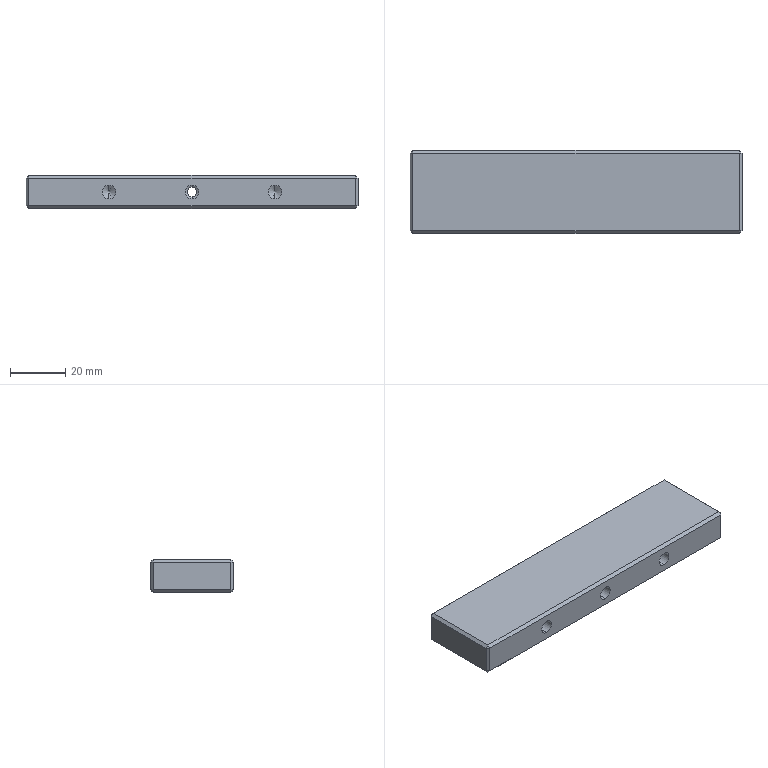Part | STEP file | 03-17 trimming upper support bracket | 1 solid | 50 faces | box 120 x 30 x 12 mm | volume 41120 mm3 | plane 26 | cylinder 12 | cone 12 | commonest cylinder face diameters 5 x12
STEP:
#1=CARTESIAN_POINT('',(35.,1.,3.5));
#2=VERTEX_POINT('',#1);
#3=CARTESIAN_POINT('',(35.,1.,8.5));
#4=VERTEX_POINT('',#3);
#5=CARTESIAN_POINT('',(35.,1.,6.));
#6=DIRECTION('',(0.,1.,0.));
#7=DIRECTION('',(0.,0.,1.));
#8=AXIS2_PLACEMENT_3D('',#5,#6,#7);
#9=CIRCLE('',#8,2.5);
#10=EDGE_CURVE('',#2,#4,#9,.T.);
#11=ORIENTED_EDGE('',*,*,#10,.F.);
#12=CARTESIAN_POINT('',(35.,15.,3.5));
#13=VERTEX_POINT('',#12);
#14=CARTESIAN_POINT('',(35.,15.,3.5));
#15=DIRECTION('',(0.,1.,0.));
#16=VECTOR('',#15,1000.);
#17=LINE('',#14,#16);
#18=EDGE_CURVE('',#2,#13,#17,.T.);
#19=ORIENTED_EDGE('',*,*,#18,.T.);
#20=CARTESIAN_POINT('',(35.,15.,8.5));
#21=VERTEX_POINT('',#20);
#22=CARTESIAN_POINT('',(35.,15.,6.));
#23=DIRECTION('',(0.,1.,0.));
#24=DIRECTION('',(0.,0.,1.));
#25=AXIS2_PLACEMENT_3D('',#22,#23,#24);
#26=CIRCLE('',#25,2.5);
#27=EDGE_CURVE('',#13,#21,#26,.T.);
#28=ORIENTED_EDGE('',*,*,#27,.T.);
#29=CARTESIAN_POINT('',(35.,15.,8.5));
#30=DIRECTION('',(0.,1.,0.));
#31=VECTOR('',#30,1000.);
#32=LINE('',#29,#31);
#33=EDGE_CURVE('',#4,#21,#32,.T.);
#34=ORIENTED_EDGE('',*,*,#33,.F.);
#35=EDGE_LOOP('',(#11,#19,#28,#34));
#36=FACE_OUTER_BOUND('',#35,.T.);
#37=CARTESIAN_POINT('',(35.,15.,6.));
#38=DIRECTION('',(0.,1.,0.));
#39=DIRECTION('',(0.,0.,1.));
#40=AXIS2_PLACEMENT_3D('',#37,#38,#39);
#41=CYLINDRICAL_SURFACE('',#40,2.5);
#42=ADVANCED_FACE('',(#36),#41,.F.);
#43=CARTESIAN_POINT('',(35.,-0.5022,6.));
#44=VERTEX_POINT('',#43);
#45=CARTESIAN_POINT('',(35.,1.,8.5));
#46=DIRECTION('',(0.,0.515,0.8572));
#47=VECTOR('',#46,1000.);
#48=LINE('',#45,#47);
#49=EDGE_CURVE('',#44,#4,#48,.T.);
#50=ORIENTED_EDGE('',*,*,#49,.F.);
#51=CARTESIAN_POINT('',(35.,1.,3.5));
#52=DIRECTION('',(0.,0.515,-0.8572));
#53=VECTOR('',#52,1000.);
#54=LINE('',#51,#53);
#55=EDGE_CURVE('',#44,#2,#54,.T.);
#56=ORIENTED_EDGE('',*,*,#55,.T.);
#57=ORIENTED_EDGE('',*,*,#10,.T.);
#58=EDGE_LOOP('',(#50,#56,#57));
#59=FACE_OUTER_BOUND('',#58,.T.);
#60=CARTESIAN_POINT('',(35.,1.,6.));
#61=DIRECTION('',(0.,1.,0.));
#62=DIRECTION('',(0.,0.,1.));
#63=AXIS2_PLACEMENT_3D('',#60,#61,#62);
#64=CONICAL_SURFACE('',#63,2.5,1.03);
#65=ADVANCED_FACE('',(#59),#64,.F.);
#66=CARTESIAN_POINT('',(0.,1.,3.5));
#67=VERTEX_POINT('',#66);
#68=CARTESIAN_POINT('',(0.,1.,8.5));
#69=VERTEX_POINT('',#68);
#70=CARTESIAN_POINT('',(0.,1.,6.));
#71=DIRECTION('',(0.,1.,0.));
#72=DIRECTION('',(0.,0.,1.));
#73=AXIS2_PLACEMENT_3D('',#70,#71,#72);
#74=CIRCLE('',#73,2.5);
#75=EDGE_CURVE('',#67,#69,#74,.T.);
#76=ORIENTED_EDGE('',*,*,#75,.F.);
#77=CARTESIAN_POINT('',(0.,15.,3.5));
#78=VERTEX_POINT('',#77);
#79=CARTESIAN_POINT('',(0.,15.,3.5));
#80=DIRECTION('',(0.,1.,0.));
#81=VECTOR('',#80,1000.);
#82=LINE('',#79,#81);
#83=EDGE_CURVE('',#67,#78,#82,.T.);
#84=ORIENTED_EDGE('',*,*,#83,.T.);
#85=CARTESIAN_POINT('',(0.,15.,8.5));
#86=VERTEX_POINT('',#85);
#87=CARTESIAN_POINT('',(0.,15.,6.));
#88=DIRECTION('',(0.,1.,0.));
#89=DIRECTION('',(0.,0.,1.));
#90=AXIS2_PLACEMENT_3D('',#87,#88,#89);
#91=CIRCLE('',#90,2.5);
#92=EDGE_CURVE('',#78,#86,#91,.T.);
#93=ORIENTED_EDGE('',*,*,#92,.T.);
#94=CARTESIAN_POINT('',(0.,15.,8.5));
#95=DIRECTION('',(0.,1.,0.));
#96=VECTOR('',#95,1000.);
#97=LINE('',#94,#96);
#98=EDGE_CURVE('',#69,#86,#97,.T.);
#99=ORIENTED_EDGE('',*,*,#98,.F.);
#100=EDGE_LOOP('',(#76,#84,#93,#99));
#101=FACE_OUTER_BOUND('',#100,.T.);
#102=CARTESIAN_POINT('',(0.,15.,6.));
#103=DIRECTION('',(0.,1.,0.));
#104=DIRECTION('',(0.,0.,1.));
#105=AXIS2_PLACEMENT_3D('',#102,#103,#104);
#106=CYLINDRICAL_SURFACE('',#105,2.5);
#107=ADVANCED_FACE('',(#101),#106,.F.);
#108=CARTESIAN_POINT('',(0.,0.5,4.332));
#109=VERTEX_POINT('',#108);
#110=CARTESIAN_POINT('',(0.,0.5,7.668));
#111=VERTEX_POINT('',#110);
#112=CARTESIAN_POINT('',(0.,0.5,6.));
#113=DIRECTION('',(0.,1.,0.));
#114=DIRECTION('',(0.,0.,1.));
#115=AXIS2_PLACEMENT_3D('',#112,#113,#114);
#116=CIRCLE('',#115,1.668);
#117=EDGE_CURVE('',#109,#111,#116,.T.);
#118=ORIENTED_EDGE('',*,*,#117,.F.);
#119=CARTESIAN_POINT('',(0.,1.,3.5));
#120=DIRECTION('',(0.,0.515,-0.8572));
#121=VECTOR('',#120,1000.);
#122=LINE('',#119,#121);
#123=EDGE_CURVE('',#109,#67,#122,.T.);
#124=ORIENTED_EDGE('',*,*,#123,.T.);
#125=ORIENTED_EDGE('',*,*,#75,.T.);
#126=CARTESIAN_POINT('',(0.,1.,8.5));
#127=DIRECTION('',(0.,0.515,0.8572));
#128=VECTOR('',#127,1000.);
#129=LINE('',#126,#128);
#130=EDGE_CURVE('',#111,#69,#129,.T.);
#131=ORIENTED_EDGE('',*,*,#130,.F.);
#132=EDGE_LOOP('',(#118,#124,#125,#131));
#133=FACE_OUTER_BOUND('',#132,.T.);
#134=CARTESIAN_POINT('',(0.,1.,6.));
#135=DIRECTION('',(0.,1.,0.));
#136=DIRECTION('',(0.,0.,1.));
#137=AXIS2_PLACEMENT_3D('',#134,#135,#136);
#138=CONICAL_SURFACE('',#137,2.5,1.03);
#139=ADVANCED_FACE('',(#133),#138,.F.);
#140=CARTESIAN_POINT('',(-35.,1.,3.5));
#141=VERTEX_POINT('',#140);
#142=CARTESIAN_POINT('',(-35.,1.,8.5));
#143=VERTEX_POINT('',#142);
#144=CARTESIAN_POINT('',(-35.,1.,6.));
#145=DIRECTION('',(0.,1.,0.));
#146=DIRECTION('',(0.,0.,1.));
#147=AXIS2_PLACEMENT_3D('',#144,#145,#146);
#148=CIRCLE('',#147,2.5);
#149=EDGE_CURVE('',#141,#143,#148,.T.);
#150=ORIENTED_EDGE('',*,*,#149,.F.);
#151=CARTESIAN_POINT('',(-35.,15.,3.5));
#152=VERTEX_POINT('',#151);
#153=CARTESIAN_POINT('',(-35.,15.,3.5));
#154=DIRECTION('',(0.,1.,0.));
#155=VECTOR('',#154,1000.);
#156=LINE('',#153,#155);
#157=EDGE_CURVE('',#141,#152,#156,.T.);
#158=ORIENTED_EDGE('',*,*,#157,.T.);
#159=CARTESIAN_POINT('',(-35.,15.,8.5));
#160=VERTEX_POINT('',#159);
#161=CARTESIAN_POINT('',(-35.,15.,6.));
#162=DIRECTION('',(0.,1.,0.));
#163=DIRECTION('',(0.,0.,1.));
#164=AXIS2_PLACEMENT_3D('',#161,#162,#163);
#165=CIRCLE('',#164,2.5);
#166=EDGE_CURVE('',#152,#160,#165,.T.);
#167=ORIENTED_EDGE('',*,*,#166,.T.);
#168=CARTESIAN_POINT('',(-35.,15.,8.5));
#169=DIRECTION('',(0.,1.,0.));
#170=VECTOR('',#169,1000.);
#171=LINE('',#168,#170);
#172=EDGE_CURVE('',#143,#160,#171,.T.);
#173=ORIENTED_EDGE('',*,*,#172,.F.);
#174=EDGE_LOOP('',(#150,#158,#167,#173));
#175=FACE_OUTER_BOUND('',#174,.T.);
#176=CARTESIAN_POINT('',(-35.,15.,6.));
#177=DIRECTION('',(0.,1.,0.));
#178=DIRECTION('',(0.,0.,1.));
#179=AXIS2_PLACEMENT_3D('',#176,#177,#178);
#180=CYLINDRICAL_SURFACE('',#179,2.5);
#181=ADVANCED_FACE('',(#175),#180,.F.);
#182=CARTESIAN_POINT('',(-35.,-0.5022,6.));
#183=VERTEX_POINT('',#182);
#184=CARTESIAN_POINT('',(-35.,1.,8.5));
#185=DIRECTION('',(0.,0.515,0.8572));
#186=VECTOR('',#185,1000.);
#187=LINE('',#184,#186);
#188=EDGE_CURVE('',#183,#143,#187,.T.);
#189=ORIENTED_EDGE('',*,*,#188,.F.);
#190=CARTESIAN_POINT('',(-35.,1.,3.5));
#191=DIRECTION('',(0.,0.515,-0.8572));
#192=VECTOR('',#191,1000.);
#193=LINE('',#190,#192);
#194=EDGE_CURVE('',#183,#141,#193,.T.);
#195=ORIENTED_EDGE('',*,*,#194,.T.);
#196=ORIENTED_EDGE('',*,*,#149,.T.);
#197=EDGE_LOOP('',(#189,#195,#196));
#198=FACE_OUTER_BOUND('',#197,.T.);
#199=CARTESIAN_POINT('',(-35.,1.,6.));
#200=DIRECTION('',(0.,1.,0.));
#201=DIRECTION('',(0.,0.,1.));
#202=AXIS2_PLACEMENT_3D('',#199,#200,#201);
#203=CONICAL_SURFACE('',#202,2.5,1.03);
#204=ADVANCED_FACE('',(#198),#203,.F.);
#205=CARTESIAN_POINT('',(30.,0.,8.5));
#206=VERTEX_POINT('',#205);
#207=CARTESIAN_POINT('',(30.,0.,3.5));
#208=VERTEX_POINT('',#207);
#209=CARTESIAN_POINT('',(30.,0.,6.));
#210=DIRECTION('',(0.,-1.,0.));
#211=DIRECTION('',(0.,0.,-1.));
#212=AXIS2_PLACEMENT_3D('',#209,#210,#211);
#213=CIRCLE('',#212,2.5);
#214=EDGE_CURVE('',#206,#208,#213,.T.);
#215=ORIENTED_EDGE('',*,*,#214,.F.);
#216=CARTESIAN_POINT('',(30.,-15.,8.5));
#217=VERTEX_POINT('',#216);
#218=CARTESIAN_POINT('',(30.,-15.,8.5));
#219=DIRECTION('',(0.,-1.,0.));
#220=VECTOR('',#219,1000.);
#221=LINE('',#218,#220);
#222=EDGE_CURVE('',#206,#217,#221,.T.);
#223=ORIENTED_EDGE('',*,*,#222,.T.);
#224=CARTESIAN_POINT('',(30.,-15.,3.5));
#225=VERTEX_POINT('',#224);
#226=CARTESIAN_POINT('',(30.,-15.,6.));
#227=DIRECTION('',(0.,-1.,0.));
#228=DIRECTION('',(0.,0.,-1.));
#229=AXIS2_PLACEMENT_3D('',#226,#227,#228);
#230=CIRCLE('',#229,2.5);
#231=EDGE_CURVE('',#217,#225,#230,.T.);
#232=ORIENTED_EDGE('',*,*,#231,.T.);
#233=CARTESIAN_POINT('',(30.,-15.,3.5));
#234=DIRECTION('',(0.,-1.,0.));
#235=VECTOR('',#234,1000.);
#236=LINE('',#233,#235);
#237=EDGE_CURVE('',#208,#225,#236,.T.);
#238=ORIENTED_EDGE('',*,*,#237,.F.);
#239=EDGE_LOOP('',(#215,#223,#232,#238));
#240=FACE_OUTER_BOUND('',#239,.T.);
#241=CARTESIAN_POINT('',(30.,-15.,6.));
#242=DIRECTION('',(0.,-1.,0.));
#243=DIRECTION('',(0.,0.,-1.));
#244=AXIS2_PLACEMENT_3D('',#241,#242,#243);
#245=CYLINDRICAL_SURFACE('',#244,2.5);
#246=ADVANCED_FACE('',(#240),#245,.F.);
#247=CARTESIAN_POINT('',(30.,1.502,6.));
#248=VERTEX_POINT('',#247);
#249=CARTESIAN_POINT('',(30.,0.,3.5));
#250=DIRECTION('',(0.,-0.515,-0.8572));
#251=VECTOR('',#250,1000.);
#252=LINE('',#249,#251);
#253=EDGE_CURVE('',#248,#208,#252,.T.);
#254=ORIENTED_EDGE('',*,*,#253,.F.);
#255=CARTESIAN_POINT('',(30.,0.,8.5));
#256=DIRECTION('',(0.,-0.515,0.8572));
#257=VECTOR('',#256,1000.);
#258=LINE('',#255,#257);
#259=EDGE_CURVE('',#248,#206,#258,.T.);
#260=ORIENTED_EDGE('',*,*,#259,.T.);
#261=ORIENTED_EDGE('',*,*,#214,.T.);
#262=EDGE_LOOP('',(#254,#260,#261));
#263=FACE_OUTER_BOUND('',#262,.T.);
#264=CARTESIAN_POINT('',(30.,0.,6.));
#265=DIRECTION('',(0.,-1.,0.));
#266=DIRECTION('',(0.,0.,-1.));
#267=AXIS2_PLACEMENT_3D('',#264,#265,#266);
#268=CONICAL_SURFACE('',#267,2.5,1.03);
#269=ADVANCED_FACE('',(#263),#268,.F.);
#270=CARTESIAN_POINT('',(0.,0.,8.5));
#271=VERTEX_POINT('',#270);
#272=CARTESIAN_POINT('',(0.,0.,3.5));
#273=VERTEX_POINT('',#272);
#274=CARTESIAN_POINT('',(0.,0.,6.));
#275=DIRECTION('',(0.,-1.,0.));
#276=DIRECTION('',(0.,0.,-1.));
#277=AXIS2_PLACEMENT_3D('',#274,#275,#276);
#278=CIRCLE('',#277,2.5);
#279=EDGE_CURVE('',#271,#273,#278,.T.);
#280=ORIENTED_EDGE('',*,*,#279,.F.);
#281=CARTESIAN_POINT('',(0.,-15.,8.5));
#282=VERTEX_POINT('',#281);
#283=CARTESIAN_POINT('',(0.,-15.,8.5));
#284=DIRECTION('',(0.,-1.,0.));
#285=VECTOR('',#284,1000.);
#286=LINE('',#283,#285);
#287=EDGE_CURVE('',#271,#282,#286,.T.);
#288=ORIENTED_EDGE('',*,*,#287,.T.);
#289=CARTESIAN_POINT('',(0.,-15.,3.5));
#290=VERTEX_POINT('',#289);
#291=CARTESIAN_POINT('',(0.,-15.,6.));
#292=DIRECTION('',(0.,-1.,0.));
#293=DIRECTION('',(0.,0.,-1.));
#294=AXIS2_PLACEMENT_3D('',#291,#292,#293);
#295=CIRCLE('',#294,2.5);
#296=EDGE_CURVE('',#282,#290,#295,.T.);
#297=ORIENTED_EDGE('',*,*,#296,.T.);
#298=CARTESIAN_POINT('',(0.,-15.,3.5));
#299=DIRECTION('',(0.,-1.,0.));
#300=VECTOR('',#299,1000.);
#301=LINE('',#298,#300);
#302=EDGE_CURVE('',#273,#290,#301,.T.);
#303=ORIENTED_EDGE('',*,*,#302,.F.);
#304=EDGE_LOOP('',(#280,#288,#297,#303));
#305=FACE_OUTER_BOUND('',#304,.T.);
#306=CARTESIAN_POINT('',(0.,-15.,6.));
#307=DIRECTION('',(0.,-1.,0.));
#308=DIRECTION('',(0.,0.,-1.));
#309=AXIS2_PLACEMENT_3D('',#306,#307,#308);
#310=CYLINDRICAL_SURFACE('',#309,2.5);
#311=ADVANCED_FACE('',(#305),#310,.F.);
#312=ORIENTED_EDGE('',*,*,#117,.T.);
#313=CARTESIAN_POINT('',(0.,0.,8.5));
#314=DIRECTION('',(0.,-0.515,0.8572));
#315=VECTOR('',#314,1000.);
#316=LINE('',#313,#315);
#317=EDGE_CURVE('',#111,#271,#316,.T.);
#318=ORIENTED_EDGE('',*,*,#317,.T.);
#319=ORIENTED_EDGE('',*,*,#279,.T.);
#320=CARTESIAN_POINT('',(0.,0.,3.5));
#321=DIRECTION('',(0.,-0.515,-0.8572));
#322=VECTOR('',#321,1000.);
#323=LINE('',#320,#322);
#324=EDGE_CURVE('',#109,#273,#323,.T.);
#325=ORIENTED_EDGE('',*,*,#324,.F.);
#326=EDGE_LOOP('',(#312,#318,#319,#325));
#327=FACE_OUTER_BOUND('',#326,.T.);
#328=CARTESIAN_POINT('',(0.,0.,6.));
#329=DIRECTION('',(0.,-1.,0.));
#330=DIRECTION('',(0.,0.,-1.));
#331=AXIS2_PLACEMENT_3D('',#328,#329,#330);
#332=CONICAL_SURFACE('',#331,2.5,1.03);
#333=ADVANCED_FACE('',(#327),#332,.F.);
#334=CARTESIAN_POINT('',(-30.,0.,8.5));
#335=VERTEX_POINT('',#334);
#336=CARTESIAN_POINT('',(-30.,0.,3.5));
#337=VERTEX_POINT('',#336);
#338=CARTESIAN_POINT('',(-30.,0.,6.));
#339=DIRECTION('',(0.,-1.,0.));
#340=DIRECTION('',(0.,0.,-1.));
#341=AXIS2_PLACEMENT_3D('',#338,#339,#340);
#342=CIRCLE('',#341,2.5);
#343=EDGE_CURVE('',#335,#337,#342,.T.);
#344=ORIENTED_EDGE('',*,*,#343,.F.);
#345=CARTESIAN_POINT('',(-30.,-15.,8.5));
#346=VERTEX_POINT('',#345);
#347=CARTESIAN_POINT('',(-30.,-15.,8.5));
#348=DIRECTION('',(0.,-1.,0.));
#349=VECTOR('',#348,1000.);
#350=LINE('',#347,#349);
#351=EDGE_CURVE('',#335,#346,#350,.T.);
#352=ORIENTED_EDGE('',*,*,#351,.T.);
#353=CARTESIAN_POINT('',(-30.,-15.,3.5));
#354=VERTEX_POINT('',#353);
#355=CARTESIAN_POINT('',(-30.,-15.,6.));
#356=DIRECTION('',(0.,-1.,0.));
#357=DIRECTION('',(0.,0.,-1.));
#358=AXIS2_PLACEMENT_3D('',#355,#356,#357);
#359=CIRCLE('',#358,2.5);
#360=EDGE_CURVE('',#346,#354,#359,.T.);
#361=ORIENTED_EDGE('',*,*,#360,.T.);
#362=CARTESIAN_POINT('',(-30.,-15.,3.5));
#363=DIRECTION('',(0.,-1.,0.));
#364=VECTOR('',#363,1000.);
#365=LINE('',#362,#364);
#366=EDGE_CURVE('',#337,#354,#365,.T.);
#367=ORIENTED_EDGE('',*,*,#366,.F.);
#368=EDGE_LOOP('',(#344,#352,#361,#367));
#369=FACE_OUTER_BOUND('',#368,.T.);
#370=CARTESIAN_POINT('',(-30.,-15.,6.));
#371=DIRECTION('',(0.,-1.,0.));
#372=DIRECTION('',(0.,0.,-1.));
#373=AXIS2_PLACEMENT_3D('',#370,#371,#372);
#374=CYLINDRICAL_SURFACE('',#373,2.5);
#375=ADVANCED_FACE('',(#369),#374,.F.);
#376=CARTESIAN_POINT('',(-30.,1.502,6.));
#377=VERTEX_POINT('',#376);
#378=CARTESIAN_POINT('',(-30.,0.,3.5));
#379=DIRECTION('',(0.,-0.515,-0.8572));
#380=VECTOR('',#379,1000.);
#381=LINE('',#378,#380);
#382=EDGE_CURVE('',#377,#337,#381,.T.);
#383=ORIENTED_EDGE('',*,*,#382,.F.);
#384=CARTESIAN_POINT('',(-30.,0.,8.5));
#385=DIRECTION('',(0.,-0.515,0.8572));
#386=VECTOR('',#385,1000.);
#387=LINE('',#384,#386);
#388=EDGE_CURVE('',#377,#335,#387,.T.);
#389=ORIENTED_EDGE('',*,*,#388,.T.);
#390=ORIENTED_EDGE('',*,*,#343,.T.);
#391=EDGE_LOOP('',(#383,#389,#390));
#392=FACE_OUTER_BOUND('',#391,.T.);
#393=CARTESIAN_POINT('',(-30.,0.,6.));
#394=DIRECTION('',(0.,-1.,0.));
#395=DIRECTION('',(0.,0.,-1.));
#396=AXIS2_PLACEMENT_3D('',#393,#394,#395);
#397=CONICAL_SURFACE('',#396,2.5,1.03);
#398=ADVANCED_FACE('',(#392),#397,.F.);
#399=CARTESIAN_POINT('',(60.,14.,1.));
#400=VERTEX_POINT('',#399);
#401=CARTESIAN_POINT('',(60.,14.,11.));
#402=VERTEX_POINT('',#401);
#403=CARTESIAN_POINT('',(60.,14.,12.));
#404=DIRECTION('',(0.,0.,1.));
#405=VECTOR('',#404,1000.);
#406=LINE('',#403,#405);
#407=EDGE_CURVE('',#400,#402,#406,.T.);
#408=ORIENTED_EDGE('',*,*,#407,.T.);
#409=CARTESIAN_POINT('',(60.,-14.,11.));
#410=VERTEX_POINT('',#409);
#411=CARTESIAN_POINT('',(60.,-15.,11.));
#412=DIRECTION('',(0.,-1.,0.));
#413=VECTOR('',#412,1000.);
#414=LINE('',#411,#413);
#415=EDGE_CURVE('',#402,#410,#414,.T.);
#416=ORIENTED_EDGE('',*,*,#415,.T.);
#417=CARTESIAN_POINT('',(60.,-14.,1.));
#418=VERTEX_POINT('',#417);
#419=CARTESIAN_POINT('',(60.,-14.,12.));
#420=DIRECTION('',(0.,0.,-1.));
#421=VECTOR('',#420,1000.);
#422=LINE('',#419,#421);
#423=EDGE_CURVE('',#410,#418,#422,.T.);
#424=ORIENTED_EDGE('',*,*,#423,.T.);
#425=CARTESIAN_POINT('',(60.,15.,1.));
#426=DIRECTION('',(0.,1.,0.));
#427=VECTOR('',#426,1000.);
#428=LINE('',#425,#427);
#429=EDGE_CURVE('',#418,#400,#428,.T.);
#430=ORIENTED_EDGE('',*,*,#429,.T.);
#431=EDGE_LOOP('',(#408,#416,#424,#430));
#432=FACE_OUTER_BOUND('',#431,.T.);
#433=CARTESIAN_POINT('',(60.,15.,12.));
#434=DIRECTION('',(-1.,0.,0.));
#435=DIRECTION('',(0.,-1.,0.));
#436=AXIS2_PLACEMENT_3D('',#433,#434,#435);
#437=PLANE('',#436);
#438=ADVANCED_FACE('',(#432),#437,.F.);
#439=CARTESIAN_POINT('',(-59.,15.,11.));
#440=VERTEX_POINT('',#439);
#441=CARTESIAN_POINT('',(59.,15.,11.));
#442=VERTEX_POINT('',#441);
#443=CARTESIAN_POINT('',(60.,15.,11.));
#444=DIRECTION('',(1.,0.,0.));
#445=VECTOR('',#444,1000.);
#446=LINE('',#443,#445);
#447=EDGE_CURVE('',#440,#442,#446,.T.);
#448=ORIENTED_EDGE('',*,*,#447,.T.);
#449=CARTESIAN_POINT('',(59.,15.,1.));
#450=VERTEX_POINT('',#449);
#451=CARTESIAN_POINT('',(59.,15.,12.));
#452=DIRECTION('',(0.,0.,-1.));
#453=VECTOR('',#452,1000.);
#454=LINE('',#451,#453);
#455=EDGE_CURVE('',#442,#450,#454,.T.);
#456=ORIENTED_EDGE('',*,*,#455,.T.);
#457=CARTESIAN_POINT('',(-59.,15.,1.));
#458=VERTEX_POINT('',#457);
#459=CARTESIAN_POINT('',(-60.,15.,1.));
#460=DIRECTION('',(-1.,0.,0.));
#461=VECTOR('',#460,1000.);
#462=LINE('',#459,#461);
#463=EDGE_CURVE('',#450,#458,#462,.T.);
#464=ORIENTED_EDGE('',*,*,#463,.T.);
#465=CARTESIAN_POINT('',(-59.,15.,12.));
#466=DIRECTION('',(0.,0.,1.));
#467=VECTOR('',#466,1000.);
#468=LINE('',#465,#467);
#469=EDGE_CURVE('',#458,#440,#468,.T.);
#470=ORIENTED_EDGE('',*,*,#469,.T.);
#471=EDGE_LOOP('',(#448,#456,#464,#470));
#472=FACE_OUTER_BOUND('',#471,.T.);
#473=CARTESIAN_POINT('',(35.,15.,6.));
#474=DIRECTION('',(0.,1.,0.));
#475=DIRECTION('',(0.,0.,1.));
#476=AXIS2_PLACEMENT_3D('',#473,#474,#475);
#477=CIRCLE('',#476,2.5);
#478=EDGE_CURVE('',#21,#13,#477,.T.);
#479=ORIENTED_EDGE('',*,*,#478,.F.);
#480=ORIENTED_EDGE('',*,*,#27,.F.);
#481=EDGE_LOOP('',(#479,#480));
#482=FACE_BOUND('',#481,.T.);
#483=CARTESIAN_POINT('',(0.,15.,6.));
#484=DIRECTION('',(0.,1.,0.));
#485=DIRECTION('',(0.,0.,1.));
#486=AXIS2_PLACEMENT_3D('',#483,#484,#485);
#487=CIRCLE('',#486,2.5);
#488=EDGE_CURVE('',#86,#78,#487,.T.);
#489=ORIENTED_EDGE('',*,*,#488,.F.);
#490=ORIENTED_EDGE('',*,*,#92,.F.);
#491=EDGE_LOOP('',(#489,#490));
#492=FACE_BOUND('',#491,.T.);
#493=CARTESIAN_POINT('',(-35.,15.,6.));
#494=DIRECTION('',(0.,1.,0.));
#495=DIRECTION('',(0.,0.,1.));
#496=AXIS2_PLACEMENT_3D('',#493,#494,#495);
#497=CIRCLE('',#496,2.5);
#498=EDGE_CURVE('',#160,#152,#497,.T.);
#499=ORIENTED_EDGE('',*,*,#498,.F.);
#500=ORIENTED_EDGE('',*,*,#166,.F.);
#501=EDGE_LOOP('',(#499,#500));
#502=FACE_BOUND('',#501,.T.);
#503=CARTESIAN_POINT('',(-60.,15.,12.));
#504=DIRECTION('',(0.,-1.,0.));
#505=DIRECTION('',(0.,0.,-1.));
#506=AXIS2_PLACEMENT_3D('',#503,#504,#505);
#507=PLANE('',#506);
#508=ADVANCED_FACE('',(#472,#482,#492,#502),#507,.F.);
#509=CARTESIAN_POINT('',(-60.,14.,1.));
#510=VERTEX_POINT('',#509);
#511=CARTESIAN_POINT('',(-60.,-14.,1.));
#512=VERTEX_POINT('',#511);
#513=CARTESIAN_POINT('',(-60.,15.,1.));
#514=DIRECTION('',(0.,-1.,0.));
#515=VECTOR('',#514,1000.);
#516=LINE('',#513,#515);
#517=EDGE_CURVE('',#510,#512,#516,.T.);
#518=ORIENTED_EDGE('',*,*,#517,.T.);
#519=CARTESIAN_POINT('',(-60.,-14.,11.));
#520=VERTEX_POINT('',#519);
#521=CARTESIAN_POINT('',(-60.,-14.,12.));
#522=DIRECTION('',(0.,0.,1.));
#523=VECTOR('',#522,1000.);
#524=LINE('',#521,#523);
#525=EDGE_CURVE('',#512,#520,#524,.T.);
#526=ORIENTED_EDGE('',*,*,#525,.T.);
#527=CARTESIAN_POINT('',(-60.,14.,11.));
#528=VERTEX_POINT('',#527);
#529=CARTESIAN_POINT('',(-60.,15.,11.));
#530=DIRECTION('',(0.,1.,0.));
#531=VECTOR('',#530,1000.);
#532=LINE('',#529,#531);
#533=EDGE_CURVE('',#520,#528,#532,.T.);
#534=ORIENTED_EDGE('',*,*,#533,.T.);
#535=CARTESIAN_POINT('',(-60.,14.,12.));
#536=DIRECTION('',(0.,0.,-1.));
#537=VECTOR('',#536,1000.);
#538=LINE('',#535,#537);
#539=EDGE_CURVE('',#528,#510,#538,.T.);
#540=ORIENTED_EDGE('',*,*,#539,.T.);
#541=EDGE_LOOP('',(#518,#526,#534,#540));
#542=FACE_OUTER_BOUND('',#541,.T.);
#543=CARTESIAN_POINT('',(-60.,15.,12.));
#544=DIRECTION('',(1.,0.,0.));
#545=DIRECTION('',(0.,1.,0.));
#546=AXIS2_PLACEMENT_3D('',#543,#544,#545);
#547=PLANE('',#546);
#548=ADVANCED_FACE('',(#542),#547,.F.);
#549=CARTESIAN_POINT('',(-59.,-15.,1.));
#550=VERTEX_POINT('',#549);
#551=CARTESIAN_POINT('',(59.,-15.,1.));
#552=VERTEX_POINT('',#551);
#553=CARTESIAN_POINT('',(-60.,-15.,1.));
#554=DIRECTION('',(1.,0.,0.));
#555=VECTOR('',#554,1000.);
#556=LINE('',#553,#555);
#557=EDGE_CURVE('',#550,#552,#556,.T.);
#558=ORIENTED_EDGE('',*,*,#557,.T.);
#559=CARTESIAN_POINT('',(59.,-15.,11.));
#560=VERTEX_POINT('',#559);
#561=CARTESIAN_POINT('',(59.,-15.,12.));
#562=DIRECTION('',(0.,0.,1.));
#563=VECTOR('',#562,1000.);
#564=LINE('',#561,#563);
#565=EDGE_CURVE('',#552,#560,#564,.T.);
#566=ORIENTED_EDGE('',*,*,#565,.T.);
#567=CARTESIAN_POINT('',(-59.,-15.,11.));
#568=VERTEX_POINT('',#567);
#569=CARTESIAN_POINT('',(-60.,-15.,11.));
#570=DIRECTION('',(-1.,0.,0.));
#571=VECTOR('',#570,1000.);
#572=LINE('',#569,#571);
#573=EDGE_CURVE('',#560,#568,#572,.T.);
#574=ORIENTED_EDGE('',*,*,#573,.T.);
#575=CARTESIAN_POINT('',(-59.,-15.,12.));
#576=DIRECTION('',(0.,0.,-1.));
#577=VECTOR('',#576,1000.);
#578=LINE('',#575,#577);
#579=EDGE_CURVE('',#568,#550,#578,.T.);
#580=ORIENTED_EDGE('',*,*,#579,.T.);
#581=EDGE_LOOP('',(#558,#566,#574,#580));
#582=FACE_OUTER_BOUND('',#581,.T.);
#583=CARTESIAN_POINT('',(30.,-15.,6.));
#584=DIRECTION('',(0.,-1.,0.));
#585=DIRECTION('',(0.,0.,-1.));
#586=AXIS2_PLACEMENT_3D('',#583,#584,#585);
#587=CIRCLE('',#586,2.5);
#588=EDGE_CURVE('',#225,#217,#587,.T.);
#589=ORIENTED_EDGE('',*,*,#588,.F.);
#590=ORIENTED_EDGE('',*,*,#231,.F.);
#591=EDGE_LOOP('',(#589,#590));
#592=FACE_BOUND('',#591,.T.);
#593=CARTESIAN_POINT('',(0.,-15.,6.));
#594=DIRECTION('',(0.,-1.,0.));
#595=DIRECTION('',(0.,0.,-1.));
#596=AXIS2_PLACEMENT_3D('',#593,#594,#595);
#597=CIRCLE('',#596,2.5);
#598=EDGE_CURVE('',#290,#282,#597,.T.);
#599=ORIENTED_EDGE('',*,*,#598,.F.);
#600=ORIENTED_EDGE('',*,*,#296,.F.);
#601=EDGE_LOOP('',(#599,#600));
#602=FACE_BOUND('',#601,.T.);
#603=CARTESIAN_POINT('',(-30.,-15.,6.));
#604=DIRECTION('',(0.,-1.,0.));
#605=DIRECTION('',(0.,0.,-1.));
#606=AXIS2_PLACEMENT_3D('',#603,#604,#605);
#607=CIRCLE('',#606,2.5);
#608=EDGE_CURVE('',#354,#346,#607,.T.);
#609=ORIENTED_EDGE('',*,*,#608,.F.);
#610=ORIENTED_EDGE('',*,*,#360,.F.);
#611=EDGE_LOOP('',(#609,#610));
#612=FACE_BOUND('',#611,.T.);
#613=CARTESIAN_POINT('',(-60.,-15.,12.));
#614=DIRECTION('',(0.,1.,0.));
#615=DIRECTION('',(0.,0.,1.));
#616=AXIS2_PLACEMENT_3D('',#613,#614,#615);
#617=PLANE('',#616);
#618=ADVANCED_FACE('',(#582,#592,#602,#612),#617,.F.);
#619=CARTESIAN_POINT('',(-59.,-14.,12.));
#620=VERTEX_POINT('',#619);
#621=CARTESIAN_POINT('',(59.,-14.,12.));
#622=VERTEX_POINT('',#621);
#623=CARTESIAN_POINT('',(60.,-14.,12.));
#624=DIRECTION('',(1.,0.,0.));
#625=VECTOR('',#624,1000.);
#626=LINE('',#623,#625);
#627=EDGE_CURVE('',#620,#622,#626,.T.);
#628=ORIENTED_EDGE('',*,*,#627,.T.);
#629=CARTESIAN_POINT('',(59.,14.,12.));
#630=VERTEX_POINT('',#629);
#631=CARTESIAN_POINT('',(59.,15.,12.));
#632=DIRECTION('',(0.,1.,0.));
#633=VECTOR('',#632,1000.);
#634=LINE('',#631,#633);
#635=EDGE_CURVE('',#622,#630,#634,.T.);
#636=ORIENTED_EDGE('',*,*,#635,.T.);
#637=CARTESIAN_POINT('',(-59.,14.,12.));
#638=VERTEX_POINT('',#637);
#639=CARTESIAN_POINT('',(-60.,14.,12.));
#640=DIRECTION('',(-1.,0.,0.));
#641=VECTOR('',#640,1000.);
#642=LINE('',#639,#641);
#643=EDGE_CURVE('',#630,#638,#642,.T.);
#644=ORIENTED_EDGE('',*,*,#643,.T.);
#645=CARTESIAN_POINT('',(-59.,-15.,12.));
#646=DIRECTION('',(0.,-1.,0.));
#647=VECTOR('',#646,1000.);
#648=LINE('',#645,#647);
#649=EDGE_CURVE('',#638,#620,#648,.T.);
#650=ORIENTED_EDGE('',*,*,#649,.T.);
#651=EDGE_LOOP('',(#628,#636,#644,#650));
#652=FACE_OUTER_BOUND('',#651,.T.);
#653=CARTESIAN_POINT('',(60.,-15.,12.));
#654=DIRECTION('',(0.,0.,1.));
#655=DIRECTION('',(1.,0.,0.));
#656=AXIS2_PLACEMENT_3D('',#653,#654,#655);
#657=PLANE('',#656);
#658=ADVANCED_FACE('',(#652),#657,.T.);
#659=CARTESIAN_POINT('',(-59.,14.,0.));
#660=VERTEX_POINT('',#659);
#661=CARTESIAN_POINT('',(59.,14.,0.));
#662=VERTEX_POINT('',#661);
#663=CARTESIAN_POINT('',(60.,14.,0.));
#664=DIRECTION('',(1.,0.,0.));
#665=VECTOR('',#664,1000.);
#666=LINE('',#663,#665);
#667=EDGE_CURVE('',#660,#662,#666,.T.);
#668=ORIENTED_EDGE('',*,*,#667,.T.);
#669=CARTESIAN_POINT('',(59.,-14.,0.));
#670=VERTEX_POINT('',#669);
#671=CARTESIAN_POINT('',(59.,-15.,0.));
#672=DIRECTION('',(0.,-1.,0.));
#673=VECTOR('',#672,1000.);
#674=LINE('',#671,#673);
#675=EDGE_CURVE('',#662,#670,#674,.T.);
#676=ORIENTED_EDGE('',*,*,#675,.T.);
#677=CARTESIAN_POINT('',(-59.,-14.,0.));
#678=VERTEX_POINT('',#677);
#679=CARTESIAN_POINT('',(60.,-14.,0.));
#680=DIRECTION('',(-1.,0.,0.));
#681=VECTOR('',#680,1000.);
#682=LINE('',#679,#681);
#683=EDGE_CURVE('',#670,#678,#682,.T.);
#684=ORIENTED_EDGE('',*,*,#683,.T.);
#685=CARTESIAN_POINT('',(-59.,-15.,0.));
#686=DIRECTION('',(0.,1.,0.));
#687=VECTOR('',#686,1000.);
#688=LINE('',#685,#687);
#689=EDGE_CURVE('',#678,#660,#688,.T.);
#690=ORIENTED_EDGE('',*,*,#689,.T.);
#691=EDGE_LOOP('',(#668,#676,#684,#690));
#692=FACE_OUTER_BOUND('',#691,.T.);
#693=CARTESIAN_POINT('',(60.,-15.,0.));
#694=DIRECTION('',(0.,0.,1.));
#695=DIRECTION('',(1.,0.,0.));
#696=AXIS2_PLACEMENT_3D('',#693,#694,#695);
#697=PLANE('',#696);
#698=ADVANCED_FACE('',(#692),#697,.F.);
#699=ORIENTED_EDGE('',*,*,#388,.F.);
#700=ORIENTED_EDGE('',*,*,#382,.T.);
#701=CARTESIAN_POINT('',(-30.,0.,6.));
#702=DIRECTION('',(0.,-1.,0.));
#703=DIRECTION('',(0.,0.,-1.));
#704=AXIS2_PLACEMENT_3D('',#701,#702,#703);
#705=CIRCLE('',#704,2.5);
#706=EDGE_CURVE('',#337,#335,#705,.T.);
#707=ORIENTED_EDGE('',*,*,#706,.T.);
#708=EDGE_LOOP('',(#699,#700,#707));
#709=FACE_OUTER_BOUND('',#708,.T.);
#710=CARTESIAN_POINT('',(-30.,0.,6.));
#711=DIRECTION('',(0.,-1.,0.));
#712=DIRECTION('',(0.,0.,-1.));
#713=AXIS2_PLACEMENT_3D('',#710,#711,#712);
#714=CONICAL_SURFACE('',#713,2.5,1.03);
#715=ADVANCED_FACE('',(#709),#714,.F.);
#716=ORIENTED_EDGE('',*,*,#351,.F.);
#717=ORIENTED_EDGE('',*,*,#706,.F.);
#718=ORIENTED_EDGE('',*,*,#366,.T.);
#719=ORIENTED_EDGE('',*,*,#608,.T.);
#720=EDGE_LOOP('',(#716,#717,#718,#719));
#721=FACE_OUTER_BOUND('',#720,.T.);
#722=CARTESIAN_POINT('',(-30.,-15.,6.));
#723=DIRECTION('',(0.,-1.,0.));
#724=DIRECTION('',(0.,0.,-1.));
#725=AXIS2_PLACEMENT_3D('',#722,#723,#724);
#726=CYLINDRICAL_SURFACE('',#725,2.5);
#727=ADVANCED_FACE('',(#721),#726,.F.);
#728=ORIENTED_EDGE('',*,*,#317,.F.);
#729=CARTESIAN_POINT('',(0.,0.5,6.));
#730=DIRECTION('',(0.,1.,0.));
#731=DIRECTION('',(0.,0.,1.));
#732=AXIS2_PLACEMENT_3D('',#729,#730,#731);
#733=CIRCLE('',#732,1.668);
#734=EDGE_CURVE('',#111,#109,#733,.T.);
#735=ORIENTED_EDGE('',*,*,#734,.T.);
#736=ORIENTED_EDGE('',*,*,#324,.T.);
#737=CARTESIAN_POINT('',(0.,0.,6.));
#738=DIRECTION('',(0.,-1.,0.));
#739=DIRECTION('',(0.,0.,-1.));
#740=AXIS2_PLACEMENT_3D('',#737,#738,#739);
#741=CIRCLE('',#740,2.5);
#742=EDGE_CURVE('',#273,#271,#741,.T.);
#743=ORIENTED_EDGE('',*,*,#742,.T.);
#744=EDGE_LOOP('',(#728,#735,#736,#743));
#745=FACE_OUTER_BOUND('',#744,.T.);
#746=CARTESIAN_POINT('',(0.,0.,6.));
#747=DIRECTION('',(0.,-1.,0.));
#748=DIRECTION('',(0.,0.,-1.));
#749=AXIS2_PLACEMENT_3D('',#746,#747,#748);
#750=CONICAL_SURFACE('',#749,2.5,1.03);
#751=ADVANCED_FACE('',(#745),#750,.F.);
#752=ORIENTED_EDGE('',*,*,#287,.F.);
#753=ORIENTED_EDGE('',*,*,#742,.F.);
#754=ORIENTED_EDGE('',*,*,#302,.T.);
#755=ORIENTED_EDGE('',*,*,#598,.T.);
#756=EDGE_LOOP('',(#752,#753,#754,#755));
#757=FACE_OUTER_BOUND('',#756,.T.);
#758=CARTESIAN_POINT('',(0.,-15.,6.));
#759=DIRECTION('',(0.,-1.,0.));
#760=DIRECTION('',(0.,0.,-1.));
#761=AXIS2_PLACEMENT_3D('',#758,#759,#760);
#762=CYLINDRICAL_SURFACE('',#761,2.5);
#763=ADVANCED_FACE('',(#757),#762,.F.);
#764=ORIENTED_EDGE('',*,*,#259,.F.);
#765=ORIENTED_EDGE('',*,*,#253,.T.);
#766=CARTESIAN_POINT('',(30.,0.,6.));
#767=DIRECTION('',(0.,-1.,0.));
#768=DIRECTION('',(0.,0.,-1.));
#769=AXIS2_PLACEMENT_3D('',#766,#767,#768);
#770=CIRCLE('',#769,2.5);
#771=EDGE_CURVE('',#208,#206,#770,.T.);
#772=ORIENTED_EDGE('',*,*,#771,.T.);
#773=EDGE_LOOP('',(#764,#765,#772));
#774=FACE_OUTER_BOUND('',#773,.T.);
#775=CARTESIAN_POINT('',(30.,0.,6.));
#776=DIRECTION('',(0.,-1.,0.));
#777=DIRECTION('',(0.,0.,-1.));
#778=AXIS2_PLACEMENT_3D('',#775,#776,#777);
#779=CONICAL_SURFACE('',#778,2.5,1.03);
#780=ADVANCED_FACE('',(#774),#779,.F.);
#781=ORIENTED_EDGE('',*,*,#222,.F.);
#782=ORIENTED_EDGE('',*,*,#771,.F.);
#783=ORIENTED_EDGE('',*,*,#237,.T.);
#784=ORIENTED_EDGE('',*,*,#588,.T.);
#785=EDGE_LOOP('',(#781,#782,#783,#784));
#786=FACE_OUTER_BOUND('',#785,.T.);
#787=CARTESIAN_POINT('',(30.,-15.,6.));
#788=DIRECTION('',(0.,-1.,0.));
#789=DIRECTION('',(0.,0.,-1.));
#790=AXIS2_PLACEMENT_3D('',#787,#788,#789);
#791=CYLINDRICAL_SURFACE('',#790,2.5);
#792=ADVANCED_FACE('',(#786),#791,.F.);
#793=ORIENTED_EDGE('',*,*,#194,.F.);
#794=ORIENTED_EDGE('',*,*,#188,.T.);
#795=CARTESIAN_POINT('',(-35.,1.,6.));
#796=DIRECTION('',(0.,1.,0.));
#797=DIRECTION('',(0.,0.,1.));
#798=AXIS2_PLACEMENT_3D('',#795,#796,#797);
#799=CIRCLE('',#798,2.5);
#800=EDGE_CURVE('',#143,#141,#799,.T.);
#801=ORIENTED_EDGE('',*,*,#800,.T.);
#802=EDGE_LOOP('',(#793,#794,#801));
#803=FACE_OUTER_BOUND('',#802,.T.);
#804=CARTESIAN_POINT('',(-35.,1.,6.));
#805=DIRECTION('',(0.,1.,0.));
#806=DIRECTION('',(0.,0.,1.));
#807=AXIS2_PLACEMENT_3D('',#804,#805,#806);
#808=CONICAL_SURFACE('',#807,2.5,1.03);
#809=ADVANCED_FACE('',(#803),#808,.F.);
#810=ORIENTED_EDGE('',*,*,#157,.F.);
#811=ORIENTED_EDGE('',*,*,#800,.F.);
#812=ORIENTED_EDGE('',*,*,#172,.T.);
#813=ORIENTED_EDGE('',*,*,#498,.T.);
#814=EDGE_LOOP('',(#810,#811,#812,#813));
#815=FACE_OUTER_BOUND('',#814,.T.);
#816=CARTESIAN_POINT('',(-35.,15.,6.));
#817=DIRECTION('',(0.,1.,0.));
#818=DIRECTION('',(0.,0.,1.));
#819=AXIS2_PLACEMENT_3D('',#816,#817,#818);
#820=CYLINDRICAL_SURFACE('',#819,2.5);
#821=ADVANCED_FACE('',(#815),#820,.F.);
#822=ORIENTED_EDGE('',*,*,#123,.F.);
#823=ORIENTED_EDGE('',*,*,#734,.F.);
#824=ORIENTED_EDGE('',*,*,#130,.T.);
#825=CARTESIAN_POINT('',(0.,1.,6.));
#826=DIRECTION('',(0.,1.,0.));
#827=DIRECTION('',(0.,0.,1.));
#828=AXIS2_PLACEMENT_3D('',#825,#826,#827);
#829=CIRCLE('',#828,2.5);
#830=EDGE_CURVE('',#69,#67,#829,.T.);
#831=ORIENTED_EDGE('',*,*,#830,.T.);
#832=EDGE_LOOP('',(#822,#823,#824,#831));
#833=FACE_OUTER_BOUND('',#832,.T.);
#834=CARTESIAN_POINT('',(0.,1.,6.));
#835=DIRECTION('',(0.,1.,0.));
#836=DIRECTION('',(0.,0.,1.));
#837=AXIS2_PLACEMENT_3D('',#834,#835,#836);
#838=CONICAL_SURFACE('',#837,2.5,1.03);
#839=ADVANCED_FACE('',(#833),#838,.F.);
#840=ORIENTED_EDGE('',*,*,#83,.F.);
#841=ORIENTED_EDGE('',*,*,#830,.F.);
#842=ORIENTED_EDGE('',*,*,#98,.T.);
#843=ORIENTED_EDGE('',*,*,#488,.T.);
#844=EDGE_LOOP('',(#840,#841,#842,#843));
#845=FACE_OUTER_BOUND('',#844,.T.);
#846=CARTESIAN_POINT('',(0.,15.,6.));
#847=DIRECTION('',(0.,1.,0.));
#848=DIRECTION('',(0.,0.,1.));
#849=AXIS2_PLACEMENT_3D('',#846,#847,#848);
#850=CYLINDRICAL_SURFACE('',#849,2.5);
#851=ADVANCED_FACE('',(#845),#850,.F.);
#852=ORIENTED_EDGE('',*,*,#55,.F.);
#853=ORIENTED_EDGE('',*,*,#49,.T.);
#854=CARTESIAN_POINT('',(35.,1.,6.));
#855=DIRECTION('',(0.,1.,0.));
#856=DIRECTION('',(0.,0.,1.));
#857=AXIS2_PLACEMENT_3D('',#854,#855,#856);
#858=CIRCLE('',#857,2.5);
#859=EDGE_CURVE('',#4,#2,#858,.T.);
#860=ORIENTED_EDGE('',*,*,#859,.T.);
#861=EDGE_LOOP('',(#852,#853,#860));
#862=FACE_OUTER_BOUND('',#861,.T.);
#863=CARTESIAN_POINT('',(35.,1.,6.));
#864=DIRECTION('',(0.,1.,0.));
#865=DIRECTION('',(0.,0.,1.));
#866=AXIS2_PLACEMENT_3D('',#863,#864,#865);
#867=CONICAL_SURFACE('',#866,2.5,1.03);
#868=ADVANCED_FACE('',(#862),#867,.F.);
#869=ORIENTED_EDGE('',*,*,#18,.F.);
#870=ORIENTED_EDGE('',*,*,#859,.F.);
#871=ORIENTED_EDGE('',*,*,#33,.T.);
#872=ORIENTED_EDGE('',*,*,#478,.T.);
#873=EDGE_LOOP('',(#869,#870,#871,#872));
#874=FACE_OUTER_BOUND('',#873,.T.);
#875=CARTESIAN_POINT('',(35.,15.,6.));
#876=DIRECTION('',(0.,1.,0.));
#877=DIRECTION('',(0.,0.,1.));
#878=AXIS2_PLACEMENT_3D('',#875,#876,#877);
#879=CYLINDRICAL_SURFACE('',#878,2.5);
#880=ADVANCED_FACE('',(#874),#879,.F.);
#881=CARTESIAN_POINT('',(-59.,-14.,0.));
#882=DIRECTION('',(0.7071,0.,-0.7071));
#883=VECTOR('',#882,1000.);
#884=LINE('',#881,#883);
#885=EDGE_CURVE('',#512,#678,#884,.T.);
#886=ORIENTED_EDGE('',*,*,#885,.F.);
#887=ORIENTED_EDGE('',*,*,#517,.F.);
#888=CARTESIAN_POINT('',(-59.,14.,0.));
#889=DIRECTION('',(-0.7071,0.,0.7071));
#890=VECTOR('',#889,1000.);
#891=LINE('',#888,#890);
#892=EDGE_CURVE('',#660,#510,#891,.T.);
#893=ORIENTED_EDGE('',*,*,#892,.F.);
#894=ORIENTED_EDGE('',*,*,#689,.F.);
#895=EDGE_LOOP('',(#886,#887,#893,#894));
#896=FACE_OUTER_BOUND('',#895,.T.);
#897=CARTESIAN_POINT('',(-60.,15.,1.));
#898=DIRECTION('',(0.7071,0.,0.7071));
#899=DIRECTION('',(0.7071,0.,-0.7071));
#900=AXIS2_PLACEMENT_3D('',#897,#898,#899);
#901=PLANE('',#900);
#902=ADVANCED_FACE('',(#896),#901,.F.);
#903=CARTESIAN_POINT('',(-59.5,-14.5,1.));
#904=DIRECTION('',(0.7071,-0.7071,0.));
#905=VECTOR('',#904,1000.);
#906=LINE('',#903,#905);
#907=EDGE_CURVE('',#512,#550,#906,.T.);
#908=ORIENTED_EDGE('',*,*,#907,.F.);
#909=ORIENTED_EDGE('',*,*,#885,.T.);
#910=CARTESIAN_POINT('',(-59.,-14.,0.));
#911=DIRECTION('',(0.,0.7071,-0.7071));
#912=VECTOR('',#911,1000.);
#913=LINE('',#910,#912);
#914=EDGE_CURVE('',#550,#678,#913,.T.);
#915=ORIENTED_EDGE('',*,*,#914,.F.);
#916=EDGE_LOOP('',(#908,#909,#915));
#917=FACE_OUTER_BOUND('',#916,.T.);
#918=CARTESIAN_POINT('',(-59.,-14.,0.));
#919=DIRECTION('',(-0.5774,-0.5774,-0.5774));
#920=DIRECTION('',(0.,0.7071,-0.7071));
#921=AXIS2_PLACEMENT_3D('',#918,#919,#920);
#922=PLANE('',#921);
#923=ADVANCED_FACE('',(#917),#922,.T.);
#924=CARTESIAN_POINT('',(-59.,14.,0.));
#925=DIRECTION('',(0.,0.7071,0.7071));
#926=VECTOR('',#925,1000.);
#927=LINE('',#924,#926);
#928=EDGE_CURVE('',#660,#458,#927,.T.);
#929=ORIENTED_EDGE('',*,*,#928,.F.);
#930=ORIENTED_EDGE('',*,*,#892,.T.);
#931=CARTESIAN_POINT('',(-59.5,14.5,1.));
#932=DIRECTION('',(-0.7071,-0.7071,0.));
#933=VECTOR('',#932,1000.);
#934=LINE('',#931,#933);
#935=EDGE_CURVE('',#458,#510,#934,.T.);
#936=ORIENTED_EDGE('',*,*,#935,.F.);
#937=EDGE_LOOP('',(#929,#930,#936));
#938=FACE_OUTER_BOUND('',#937,.T.);
#939=CARTESIAN_POINT('',(-59.,14.,0.));
#940=DIRECTION('',(-0.5774,0.5774,-0.5774));
#941=DIRECTION('',(0.,0.7071,0.7071));
#942=AXIS2_PLACEMENT_3D('',#939,#940,#941);
#943=PLANE('',#942);
#944=ADVANCED_FACE('',(#938),#943,.T.);
#945=ORIENTED_EDGE('',*,*,#914,.T.);
#946=ORIENTED_EDGE('',*,*,#683,.F.);
#947=CARTESIAN_POINT('',(59.,-14.,0.));
#948=DIRECTION('',(0.,0.7071,-0.7071));
#949=VECTOR('',#948,1000.);
#950=LINE('',#947,#949);
#951=EDGE_CURVE('',#552,#670,#950,.T.);
#952=ORIENTED_EDGE('',*,*,#951,.F.);
#953=ORIENTED_EDGE('',*,*,#557,.F.);
#954=EDGE_LOOP('',(#945,#946,#952,#953));
#955=FACE_OUTER_BOUND('',#954,.T.);
#956=CARTESIAN_POINT('',(-60.,-15.,1.));
#957=DIRECTION('',(0.,0.7071,0.7071));
#958=DIRECTION('',(0.,-0.7071,0.7071));
#959=AXIS2_PLACEMENT_3D('',#956,#957,#958);
#960=PLANE('',#959);
#961=ADVANCED_FACE('',(#955),#960,.F.);
#962=ORIENTED_EDGE('',*,*,#907,.T.);
#963=ORIENTED_EDGE('',*,*,#579,.F.);
#964=CARTESIAN_POINT('',(-59.,-15.,11.));
#965=DIRECTION('',(0.7071,-0.7071,0.));
#966=VECTOR('',#965,1000.);
#967=LINE('',#964,#966);
#968=EDGE_CURVE('',#520,#568,#967,.T.);
#969=ORIENTED_EDGE('',*,*,#968,.F.);
#970=ORIENTED_EDGE('',*,*,#525,.F.);
#971=EDGE_LOOP('',(#962,#963,#969,#970));
#972=FACE_OUTER_BOUND('',#971,.T.);
#973=CARTESIAN_POINT('',(-59.,-15.,12.));
#974=DIRECTION('',(0.7071,0.7071,0.));
#975=DIRECTION('',(-0.7071,0.7071,0.));
#976=AXIS2_PLACEMENT_3D('',#973,#974,#975);
#977=PLANE('',#976);
#978=ADVANCED_FACE('',(#972),#977,.F.);
#979=CARTESIAN_POINT('',(-59.5,14.,11.5));
#980=DIRECTION('',(0.7071,0.,0.7071));
#981=VECTOR('',#980,1000.);
#982=LINE('',#979,#981);
#983=EDGE_CURVE('',#528,#638,#982,.T.);
#984=ORIENTED_EDGE('',*,*,#983,.F.);
#985=ORIENTED_EDGE('',*,*,#533,.F.);
#986=CARTESIAN_POINT('',(-59.5,-14.,11.5));
#987=DIRECTION('',(-0.7071,0.,-0.7071));
#988=VECTOR('',#987,1000.);
#989=LINE('',#986,#988);
#990=EDGE_CURVE('',#620,#520,#989,.T.);
#991=ORIENTED_EDGE('',*,*,#990,.F.);
#992=ORIENTED_EDGE('',*,*,#649,.F.);
#993=EDGE_LOOP('',(#984,#985,#991,#992));
#994=FACE_OUTER_BOUND('',#993,.T.);
#995=CARTESIAN_POINT('',(-59.,-15.,12.));
#996=DIRECTION('',(-0.7071,0.,0.7071));
#997=DIRECTION('',(0.7071,0.,0.7071));
#998=AXIS2_PLACEMENT_3D('',#995,#996,#997);
#999=PLANE('',#998);
#1000=ADVANCED_FACE('',(#994),#999,.T.);
#1001=ORIENTED_EDGE('',*,*,#935,.T.);
#1002=ORIENTED_EDGE('',*,*,#539,.F.);
#1003=CARTESIAN_POINT('',(-59.,15.,11.));
#1004=DIRECTION('',(-0.7071,-0.7071,0.));
#1005=VECTOR('',#1004,1000.);
#1006=LINE('',#1003,#1005);
#1007=EDGE_CURVE('',#440,#528,#1006,.T.);
#1008=ORIENTED_EDGE('',*,*,#1007,.F.);
#1009=ORIENTED_EDGE('',*,*,#469,.F.);
#1010=EDGE_LOOP('',(#1001,#1002,#1008,#1009));
#1011=FACE_OUTER_BOUND('',#1010,.T.);
#1012=CARTESIAN_POINT('',(-60.,14.,12.));
#1013=DIRECTION('',(0.7071,-0.7071,0.));
#1014=DIRECTION('',(0.7071,0.7071,0.));
#1015=AXIS2_PLACEMENT_3D('',#1012,#1013,#1014);
#1016=PLANE('',#1015);
#1017=ADVANCED_FACE('',(#1011),#1016,.F.);
#1018=ORIENTED_EDGE('',*,*,#928,.T.);
#1019=ORIENTED_EDGE('',*,*,#463,.F.);
#1020=CARTESIAN_POINT('',(59.,15.,1.));
#1021=DIRECTION('',(0.,0.7071,0.7071));
#1022=VECTOR('',#1021,1000.);
#1023=LINE('',#1020,#1022);
#1024=EDGE_CURVE('',#662,#450,#1023,.T.);
#1025=ORIENTED_EDGE('',*,*,#1024,.F.);
#1026=ORIENTED_EDGE('',*,*,#667,.F.);
#1027=EDGE_LOOP('',(#1018,#1019,#1025,#1026));
#1028=FACE_OUTER_BOUND('',#1027,.T.);
#1029=CARTESIAN_POINT('',(-60.,15.,1.));
#1030=DIRECTION('',(0.,-0.7071,0.7071));
#1031=DIRECTION('',(0.,-0.7071,-0.7071));
#1032=AXIS2_PLACEMENT_3D('',#1029,#1030,#1031);
#1033=PLANE('',#1032);
#1034=ADVANCED_FACE('',(#1028),#1033,.F.);
#1035=CARTESIAN_POINT('',(59.,-14.,0.));
#1036=DIRECTION('',(0.7071,0.,0.7071));
#1037=VECTOR('',#1036,1000.);
#1038=LINE('',#1035,#1037);
#1039=EDGE_CURVE('',#670,#418,#1038,.T.);
#1040=ORIENTED_EDGE('',*,*,#1039,.F.);
#1041=ORIENTED_EDGE('',*,*,#675,.F.);
#1042=CARTESIAN_POINT('',(59.5,14.,0.5));
#1043=DIRECTION('',(-0.7071,0.,-0.7071));
#1044=VECTOR('',#1043,1000.);
#1045=LINE('',#1042,#1044);
#1046=EDGE_CURVE('',#400,#662,#1045,.T.);
#1047=ORIENTED_EDGE('',*,*,#1046,.F.);
#1048=ORIENTED_EDGE('',*,*,#429,.F.);
#1049=EDGE_LOOP('',(#1040,#1041,#1047,#1048));
#1050=FACE_OUTER_BOUND('',#1049,.T.);
#1051=CARTESIAN_POINT('',(60.,15.,1.));
#1052=DIRECTION('',(-0.7071,0.,0.7071));
#1053=DIRECTION('',(0.7071,0.,0.7071));
#1054=AXIS2_PLACEMENT_3D('',#1051,#1052,#1053);
#1055=PLANE('',#1054);
#1056=ADVANCED_FACE('',(#1050),#1055,.F.);
#1057=ORIENTED_EDGE('',*,*,#951,.T.);
#1058=ORIENTED_EDGE('',*,*,#1039,.T.);
#1059=CARTESIAN_POINT('',(59.5,-14.5,1.));
#1060=DIRECTION('',(0.7071,0.7071,0.));
#1061=VECTOR('',#1060,1000.);
#1062=LINE('',#1059,#1061);
#1063=EDGE_CURVE('',#552,#418,#1062,.T.);
#1064=ORIENTED_EDGE('',*,*,#1063,.F.);
#1065=EDGE_LOOP('',(#1057,#1058,#1064));
#1066=FACE_OUTER_BOUND('',#1065,.T.);
#1067=CARTESIAN_POINT('',(59.,-14.,0.));
#1068=DIRECTION('',(0.5774,-0.5774,-0.5774));
#1069=DIRECTION('',(0.7071,0.7071,0.));
#1070=AXIS2_PLACEMENT_3D('',#1067,#1068,#1069);
#1071=PLANE('',#1070);
#1072=ADVANCED_FACE('',(#1066),#1071,.T.);
#1073=ORIENTED_EDGE('',*,*,#990,.T.);
#1074=ORIENTED_EDGE('',*,*,#968,.T.);
#1075=CARTESIAN_POINT('',(-59.,-15.,11.));
#1076=DIRECTION('',(0.,-0.7071,-0.7071));
#1077=VECTOR('',#1076,1000.);
#1078=LINE('',#1075,#1077);
#1079=EDGE_CURVE('',#620,#568,#1078,.T.);
#1080=ORIENTED_EDGE('',*,*,#1079,.F.);
#1081=EDGE_LOOP('',(#1073,#1074,#1080));
#1082=FACE_OUTER_BOUND('',#1081,.T.);
#1083=CARTESIAN_POINT('',(-59.,-15.,11.));
#1084=DIRECTION('',(-0.5774,-0.5774,0.5774));
#1085=DIRECTION('',(0.,-0.7071,-0.7071));
#1086=AXIS2_PLACEMENT_3D('',#1083,#1084,#1085);
#1087=PLANE('',#1086);
#1088=ADVANCED_FACE('',(#1082),#1087,.T.);
#1089=ORIENTED_EDGE('',*,*,#1007,.T.);
#1090=ORIENTED_EDGE('',*,*,#983,.T.);
#1091=CARTESIAN_POINT('',(-59.,15.,11.));
#1092=DIRECTION('',(0.,-0.7071,0.7071));
#1093=VECTOR('',#1092,1000.);
#1094=LINE('',#1091,#1093);
#1095=EDGE_CURVE('',#440,#638,#1094,.T.);
#1096=ORIENTED_EDGE('',*,*,#1095,.F.);
#1097=EDGE_LOOP('',(#1089,#1090,#1096));
#1098=FACE_OUTER_BOUND('',#1097,.T.);
#1099=CARTESIAN_POINT('',(-59.,15.,11.));
#1100=DIRECTION('',(-0.5774,0.5774,0.5774));
#1101=DIRECTION('',(0.,-0.7071,0.7071));
#1102=AXIS2_PLACEMENT_3D('',#1099,#1100,#1101);
#1103=PLANE('',#1102);
#1104=ADVANCED_FACE('',(#1098),#1103,.T.);
#1105=ORIENTED_EDGE('',*,*,#1046,.T.);
#1106=ORIENTED_EDGE('',*,*,#1024,.T.);
#1107=CARTESIAN_POINT('',(59.,15.,1.));
#1108=DIRECTION('',(-0.7071,0.7071,0.));
#1109=VECTOR('',#1108,1000.);
#1110=LINE('',#1107,#1109);
#1111=EDGE_CURVE('',#400,#450,#1110,.T.);
#1112=ORIENTED_EDGE('',*,*,#1111,.F.);
#1113=EDGE_LOOP('',(#1105,#1106,#1112));
#1114=FACE_OUTER_BOUND('',#1113,.T.);
#1115=CARTESIAN_POINT('',(59.,15.,1.));
#1116=DIRECTION('',(0.5774,0.5774,-0.5774));
#1117=DIRECTION('',(-0.7071,0.7071,0.));
#1118=AXIS2_PLACEMENT_3D('',#1115,#1116,#1117);
#1119=PLANE('',#1118);
#1120=ADVANCED_FACE('',(#1114),#1119,.T.);
#1121=ORIENTED_EDGE('',*,*,#1063,.T.);
#1122=ORIENTED_EDGE('',*,*,#423,.F.);
#1123=CARTESIAN_POINT('',(60.,-14.,11.));
#1124=DIRECTION('',(0.7071,0.7071,0.));
#1125=VECTOR('',#1124,1000.);
#1126=LINE('',#1123,#1125);
#1127=EDGE_CURVE('',#560,#410,#1126,.T.);
#1128=ORIENTED_EDGE('',*,*,#1127,.F.);
#1129=ORIENTED_EDGE('',*,*,#565,.F.);
#1130=EDGE_LOOP('',(#1121,#1122,#1128,#1129));
#1131=FACE_OUTER_BOUND('',#1130,.T.);
#1132=CARTESIAN_POINT('',(60.,-14.,12.));
#1133=DIRECTION('',(-0.7071,0.7071,0.));
#1134=DIRECTION('',(-0.7071,-0.7071,0.));
#1135=AXIS2_PLACEMENT_3D('',#1132,#1133,#1134);
#1136=PLANE('',#1135);
#1137=ADVANCED_FACE('',(#1131),#1136,.F.);
#1138=ORIENTED_EDGE('',*,*,#1079,.T.);
#1139=ORIENTED_EDGE('',*,*,#573,.F.);
#1140=CARTESIAN_POINT('',(59.,-14.5,11.5));
#1141=DIRECTION('',(0.,-0.7071,-0.7071));
#1142=VECTOR('',#1141,1000.);
#1143=LINE('',#1140,#1142);
#1144=EDGE_CURVE('',#622,#560,#1143,.T.);
#1145=ORIENTED_EDGE('',*,*,#1144,.F.);
#1146=ORIENTED_EDGE('',*,*,#627,.F.);
#1147=EDGE_LOOP('',(#1138,#1139,#1145,#1146));
#1148=FACE_OUTER_BOUND('',#1147,.T.);
#1149=CARTESIAN_POINT('',(60.,-14.,12.));
#1150=DIRECTION('',(0.,-0.7071,0.7071));
#1151=DIRECTION('',(0.,-0.7071,-0.7071));
#1152=AXIS2_PLACEMENT_3D('',#1149,#1150,#1151);
#1153=PLANE('',#1152);
#1154=ADVANCED_FACE('',(#1148),#1153,.T.);
#1155=ORIENTED_EDGE('',*,*,#1095,.T.);
#1156=ORIENTED_EDGE('',*,*,#643,.F.);
#1157=CARTESIAN_POINT('',(59.,14.,12.));
#1158=DIRECTION('',(0.,-0.7071,0.7071));
#1159=VECTOR('',#1158,1000.);
#1160=LINE('',#1157,#1159);
#1161=EDGE_CURVE('',#442,#630,#1160,.T.);
#1162=ORIENTED_EDGE('',*,*,#1161,.F.);
#1163=ORIENTED_EDGE('',*,*,#447,.F.);
#1164=EDGE_LOOP('',(#1155,#1156,#1162,#1163));
#1165=FACE_OUTER_BOUND('',#1164,.T.);
#1166=CARTESIAN_POINT('',(60.,14.,12.));
#1167=DIRECTION('',(0.,0.7071,0.7071));
#1168=DIRECTION('',(0.,-0.7071,0.7071));
#1169=AXIS2_PLACEMENT_3D('',#1166,#1167,#1168);
#1170=PLANE('',#1169);
#1171=ADVANCED_FACE('',(#1165),#1170,.T.);
#1172=ORIENTED_EDGE('',*,*,#1111,.T.);
#1173=ORIENTED_EDGE('',*,*,#455,.F.);
#1174=CARTESIAN_POINT('',(59.5,14.5,11.));
#1175=DIRECTION('',(-0.7071,0.7071,0.));
#1176=VECTOR('',#1175,1000.);
#1177=LINE('',#1174,#1176);
#1178=EDGE_CURVE('',#402,#442,#1177,.T.);
#1179=ORIENTED_EDGE('',*,*,#1178,.F.);
#1180=ORIENTED_EDGE('',*,*,#407,.F.);
#1181=EDGE_LOOP('',(#1172,#1173,#1179,#1180));
#1182=FACE_OUTER_BOUND('',#1181,.T.);
#1183=CARTESIAN_POINT('',(59.,15.,12.));
#1184=DIRECTION('',(-0.7071,-0.7071,0.));
#1185=DIRECTION('',(0.7071,-0.7071,0.));
#1186=AXIS2_PLACEMENT_3D('',#1183,#1184,#1185);
#1187=PLANE('',#1186);
#1188=ADVANCED_FACE('',(#1182),#1187,.F.);
#1189=ORIENTED_EDGE('',*,*,#1144,.T.);
#1190=ORIENTED_EDGE('',*,*,#1127,.T.);
#1191=CARTESIAN_POINT('',(60.,-14.,11.));
#1192=DIRECTION('',(0.7071,0.,-0.7071));
#1193=VECTOR('',#1192,1000.);
#1194=LINE('',#1191,#1193);
#1195=EDGE_CURVE('',#622,#410,#1194,.T.);
#1196=ORIENTED_EDGE('',*,*,#1195,.F.);
#1197=EDGE_LOOP('',(#1189,#1190,#1196));
#1198=FACE_OUTER_BOUND('',#1197,.T.);
#1199=CARTESIAN_POINT('',(60.,-14.,11.));
#1200=DIRECTION('',(0.5774,-0.5774,0.5774));
#1201=DIRECTION('',(0.7071,0.,-0.7071));
#1202=AXIS2_PLACEMENT_3D('',#1199,#1200,#1201);
#1203=PLANE('',#1202);
#1204=ADVANCED_FACE('',(#1198),#1203,.T.);
#1205=ORIENTED_EDGE('',*,*,#1178,.T.);
#1206=ORIENTED_EDGE('',*,*,#1161,.T.);
#1207=CARTESIAN_POINT('',(59.,14.,12.));
#1208=DIRECTION('',(-0.7071,0.,0.7071));
#1209=VECTOR('',#1208,1000.);
#1210=LINE('',#1207,#1209);
#1211=EDGE_CURVE('',#402,#630,#1210,.T.);
#1212=ORIENTED_EDGE('',*,*,#1211,.F.);
#1213=EDGE_LOOP('',(#1205,#1206,#1212));
#1214=FACE_OUTER_BOUND('',#1213,.T.);
#1215=CARTESIAN_POINT('',(59.,14.,12.));
#1216=DIRECTION('',(0.5774,0.5774,0.5774));
#1217=DIRECTION('',(0.,-0.7071,0.7071));
#1218=AXIS2_PLACEMENT_3D('',#1215,#1216,#1217);
#1219=PLANE('',#1218);
#1220=ADVANCED_FACE('',(#1214),#1219,.T.);
#1221=ORIENTED_EDGE('',*,*,#1195,.T.);
#1222=ORIENTED_EDGE('',*,*,#415,.F.);
#1223=ORIENTED_EDGE('',*,*,#1211,.T.);
#1224=ORIENTED_EDGE('',*,*,#635,.F.);
#1225=EDGE_LOOP('',(#1221,#1222,#1223,#1224));
#1226=FACE_OUTER_BOUND('',#1225,.T.);
#1227=CARTESIAN_POINT('',(59.,-15.,12.));
#1228=DIRECTION('',(0.7071,0.,0.7071));
#1229=DIRECTION('',(0.7071,0.,-0.7071));
#1230=AXIS2_PLACEMENT_3D('',#1227,#1228,#1229);
#1231=PLANE('',#1230);
#1232=ADVANCED_FACE('',(#1226),#1231,.T.);
#1233=CLOSED_SHELL('',(#42,#65,#107,#139,#181,#204,#246,#269,#311,#333,#375,#398,#438,#508,#548,#618,#658,#698,#715,#727,#751,#763,#780,#792,#809,#821,#839,#851,#868,#880,#902,#923,#944,#961,#978,#1000,#1017,#1034,#1056,#1072,#1088,#1104,#1120,#1137,#1154,#1171,#1188,#1204,#1220,#1232));
#1234=MANIFOLD_SOLID_BREP('',#1233);
#1235=CARTESIAN_POINT('',(0.,0.,0.));
#1236=DIRECTION('',(0.,0.,1.));
#1237=DIRECTION('',(1.,0.,0.));
#1238=AXIS2_PLACEMENT_3D('',#1235,#1236,#1237);
#1239=(LENGTH_UNIT()NAMED_UNIT(*)SI_UNIT(.MILLI.,.METRE.));
#1240=UNCERTAINTY_MEASURE_WITH_UNIT(LENGTH_MEASURE(0.00001),#1239,'','');
#1241=(NAMED_UNIT(*)PLANE_ANGLE_UNIT()SI_UNIT($,.RADIAN.));
#1242=(NAMED_UNIT(*)SI_UNIT($,.STERADIAN.)SOLID_ANGLE_UNIT());
#1243=(GEOMETRIC_REPRESENTATION_CONTEXT(3)GLOBAL_UNCERTAINTY_ASSIGNED_CONTEXT((#1240))GLOBAL_UNIT_ASSIGNED_CONTEXT((#1239,#1241,#1242))REPRESENTATION_CONTEXT('',''));
#1244=ADVANCED_BREP_SHAPE_REPRESENTATION('',(#1234,#1238),#1243);